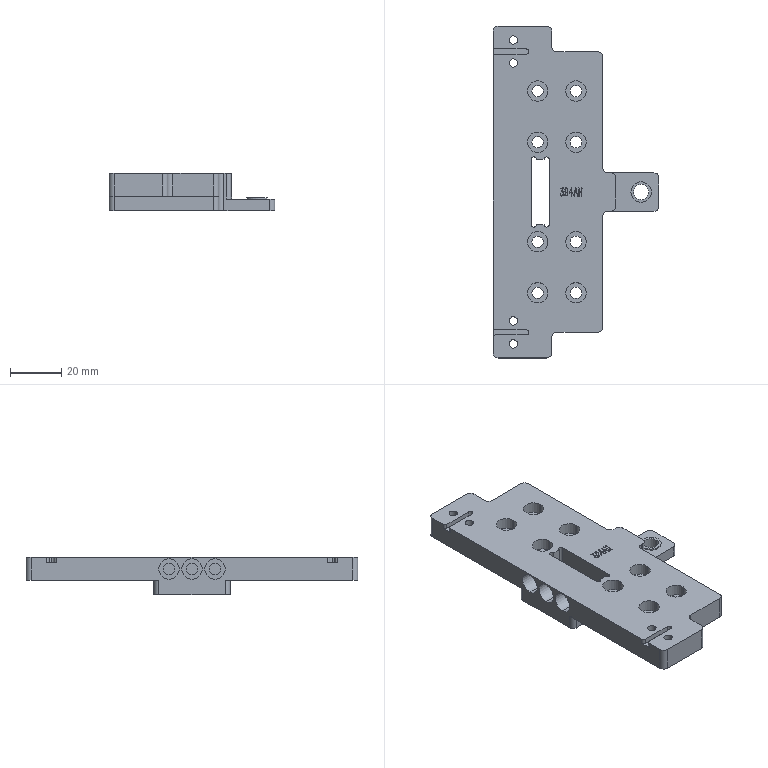NC program | NX | posted with a generic post | part box 65 x 130 x 14.5 mm
Lines 11007 to 11541 of 11541:
(PLANAR_MILL_COPY_COPY_COPY_COPY_COPY_COPY_1_COPY , TOOL : D6A45)
N21958 T01 M6
N21960 G54
N21962 G17 G0 G90 X-0.428 Y-26.291 B0. C0. S9500 M3
N21964 G43 Z30. H1
N21966 Z0.5
N21968 G94 G1 Z-1. F1250.
N21970 X-0.866 Y-27.1
N21972 G3 X0. Y-27.6 R1.
N21974 X2.1 Y-25.5 R2.1
N21976 X0. Y-27.6 R-2.1
N21978 X0.866 Y-27.1 R1.
N21980 G1 X0.428 Y-26.291
N21982 Z0.5
N21984 G0 Z30.
N21986 X-17.1 Y9.73
N21988 Z0.5
N21990 G1 Z-1.
N21992 X-16.4 Y10.134
N21994 G3 X-15.9 Y11. R1.
N21996 G1 Y30.5
N21998 G2 X-13. Y33.4 R2.9
N22000 G1 X13.
N22002 G2 X15.9 Y30.5 R2.9
N22004 G1 Y-8.5
N22006 G2 X13. Y-11.4 R2.9
N22008 G1 X9.5
N22010 G3 X8.4 Y-12.5 R1.1
N22012 G1 Y-30.5
N22014 G2 X5.5 Y-33.4 R2.9
N22016 G1 X-5.5
N22018 G2 X-8.4 Y-30.5 R2.9
N22020 G1 Y-12.5
N22022 G3 X-9.5 Y-11.4 R1.1
N22024 G1 X-13.
N22026 G2 X-15.9 Y-8.5 R2.9
N22028 G1 Y11.
N22030 G3 X-16.4 Y11.866 R1.
N22032 G1 X-17.1 Y12.27
N22034 Z0.5
N22036 G0 Z30.
N22038 X1.27 Y15.4
N22040 Z0.5
N22042 G1 Z-1.
N22044 X0.866 Y16.1
N22046 G3 X0. Y16.6 R1.
N22048 G1 X-12.75
N22050 G3 X-12.759 Y16.4 R0.1
N22052 G2 X-11.85 Y15.405 R1.
N22054 G1 Y12.595
N22056 G2 X-12.759 Y11.6 R1.
N22058 G3 X-12.75 Y11.4 R0.1
N22060 G1 X12.75
N22062 G3 X12.759 Y11.6 R0.1
N22064 G2 X11.85 Y12.595 R1.
N22066 G1 Y15.405
N22068 G2 X12.759 Y16.4 R1.
N22070 G3 X12.75 Y16.6 R0.1
N22072 G1 X0.
N22074 G3 X-0.866 Y16.1 R1.
N22076 G1 X-1.27 Y15.4
N22078 Z0.5
N22080 G0 Z30.
(PLANAR_MILL_COPY_COPY_COPY_COPY_COPY_COPY_1_COPY_COPY , TOOL : D6A45)
N22082 X59.924 Y23.874
N22084 Z-5.
N22086 G1 X60.052 Y23.948 Z-5.04
N22088 X60.25 Y24.286 Z-5.144
N22090 Y24.714 Z-5.259
N22092 X60.052 Y25.052 Z-5.364
N22094 X59.714 Y25.25 Z-5.469
N22096 X59.286 Z-5.584
N22098 X58.948 Y25.052 Z-5.689
N22100 X58.75 Y24.714 Z-5.794
N22102 Y24.286 Z-5.908
N22104 X58.948 Y23.948 Z-6.013
N22106 X59.286 Y23.75 Z-6.118
N22108 X59.714 Z-6.233
N22110 X60.052 Y23.948 Z-6.338
N22112 X60.25 Y24.286 Z-6.443
N22114 Y24.5 Z-6.5
N22116 G3 X59.5 Y25.25 R0.75
N22118 X60.25 Y24.5 R-0.75
N22120 X60. Y24.933 R0.5
N22122 G1 Z-5.
N22124 G0 Z30.
N22126 X51.126 Y24.924
N22128 Z-5.
N22130 G1 X51.052 Y25.052 Z-5.04
N22132 X50.714 Y25.25 Z-5.144
N22134 X50.286 Z-5.259
N22136 X49.948 Y25.052 Z-5.364
N22138 X49.75 Y24.714 Z-5.469
N22140 Y24.286 Z-5.584
N22142 X49.948 Y23.948 Z-5.689
N22144 X50.286 Y23.75 Z-5.794
N22146 X50.714 Z-5.908
N22148 X51.052 Y23.948 Z-6.013
N22150 X51.25 Y24.286 Z-6.118
N22152 Y24.714 Z-6.233
N22154 X51.052 Y25.052 Z-6.338
N22156 X50.714 Y25.25 Z-6.443
N22158 X50.5 Z-6.5
N22160 G3 X49.75 Y24.5 R0.75
N22162 X50.5 Y25.25 R-0.75
N22164 X50.067 Y25. R0.5
N22166 G1 Z-5.
N22168 G0 Z30.
N22170 X17.963 Y35.
N22172 Z-5.
N22174 G1 Z-6.5
N22176 X17.642 Y34.399
N22178 G3 X17.673 Y33.4 R1.
N22180 G1 X63.
N22182 G2 X65.9 Y30.5 R2.9
N22184 G1 Y11.5
N22186 G2 X63. Y8.6 R2.9
N22188 G1 X57.
N22190 G3 X55.9 Y7.5 R1.1
N22192 G1 Y-8.5
N22194 G2 X53. Y-11.4 R2.9
N22196 G1 X43.1
N22198 G2 X42.1 Y-10.4 R1.
N22200 G1 Y29.5
N22202 X42.113 Y29.565
N22204 X42.065 Y29.613
N22206 X42. Y29.6
N22208 X18.5
N22210 G3 X19. Y28.734 R1.
N22212 G1 X19.7 Y28.33
N22214 Z-5.
N22216 G0 Z30.
N22218 X-19.7
N22220 Z-5.
N22222 G1 Z-6.5
N22224 X-19. Y28.734
N22226 G3 X-18.5 Y29.6 R1.
N22228 G1 X-42.
N22230 X-42.065 Y29.613
N22232 X-42.113 Y29.565
N22234 X-42.1 Y29.5
N22236 Y-10.4
N22238 G2 X-43.1 Y-11.4 R1.
N22240 G1 X-53.
N22242 G2 X-55.9 Y-8.5 R2.9
N22244 G1 Y7.5
N22246 G3 X-57. Y8.6 R1.1
N22248 G1 X-63.
N22250 G2 X-65.9 Y11.5 R2.9
N22252 G1 Y30.5
N22254 G2 X-63. Y33.4 R2.9
N22256 G1 X-17.673
N22258 G3 X-17.642 Y34.399 R1.
N22260 G1 X-17.963 Y35.
N22262 Z-5.
N22264 G0 Z30.
N22266 X-49.874 Y24.924
N22268 Z-5.
N22270 G1 X-49.948 Y25.052 Z-5.04
N22272 X-50.286 Y25.25 Z-5.144
N22274 X-50.714 Z-5.259
N22276 X-51.052 Y25.052 Z-5.364
N22278 X-51.25 Y24.714 Z-5.469
N22280 Y24.286 Z-5.584
N22282 X-51.052 Y23.948 Z-5.689
N22284 X-50.714 Y23.75 Z-5.794
N22286 X-50.286 Z-5.908
N22288 X-49.948 Y23.948 Z-6.013
N22290 X-49.75 Y24.286 Z-6.118
N22292 Y24.714 Z-6.233
N22294 X-49.948 Y25.052 Z-6.338
N22296 X-50.286 Y25.25 Z-6.443
N22298 X-50.5 Z-6.5
N22300 G3 X-51.25 Y24.5 R0.75
N22302 X-50.5 Y25.25 R-0.75
N22304 X-50.933 Y25. R0.5
N22306 G1 Z-5.
N22308 G0 Z30.
N22310 X-59.924 Y25.126
N22312 Z-5.
N22314 G1 X-60.052 Y25.052 Z-5.04
N22316 X-60.25 Y24.714 Z-5.144
N22318 Y24.286 Z-5.259
N22320 X-60.052 Y23.948 Z-5.364
N22322 X-59.714 Y23.75 Z-5.469
N22324 X-59.286 Z-5.584
N22326 X-58.948 Y23.948 Z-5.689
N22328 X-58.75 Y24.286 Z-5.794
N22330 Y24.714 Z-5.908
N22332 X-58.948 Y25.052 Z-6.013
N22334 X-59.286 Y25.25 Z-6.118
N22336 X-59.714 Z-6.233
N22338 X-60.052 Y25.052 Z-6.338
N22340 X-60.25 Y24.714 Z-6.443
N22342 Y24.5 Z-6.5
N22344 G3 X-59.5 Y23.75 R0.75
N22346 X-60.25 Y24.5 R-0.75
N22348 X-60. Y24.067 R0.5
N22350 G1 Z-5.
N22352 G0 Z30.
(PLANAR_MILL_COPY_COPY_COPY_COPY_COPY_COPY_1_COPY_COPY_COPY , TOOL : D6A45)
N22354 X-38.408 Y0.761
N22356 Z-7.5
N22358 G1 X-38.524 Y0.976 Z-7.565
N22360 X-39.214 Y1.35 Z-7.776
N22362 X-39.5 Z-7.852
N22364 X-39.214 Z-7.929
N22366 X-38.524 Y0.976 Z-8.139
N22368 X-38.15 Y0.286 Z-8.349
N22370 Y-0.286 Z-8.503
N22372 X-38.524 Y-0.976 Z-8.713
N22374 X-39.214 Y-1.35 Z-8.923
N22376 X-39.5 Z-9.
N22378 G3 X-38.15 Y0. R1.35
N22380 X-39.5 Y1.35 R1.35
N22382 X-39. Y0.484 R1.
N22384 G1 Z-7.5
N22386 G0 Z30.
N22388 X-38.408 Y15.761
N22390 Z-7.5
N22392 G1 X-38.524 Y15.976 Z-7.565
N22394 X-39.214 Y16.35 Z-7.776
N22396 X-39.5 Z-7.852
N22398 X-39.214 Z-7.929
N22400 X-38.524 Y15.976 Z-8.139
N22402 X-38.15 Y15.286 Z-8.349
N22404 Y14.714 Z-8.503
N22406 X-38.524 Y14.024 Z-8.713
N22408 X-39.214 Y13.65 Z-8.923
N22410 X-39.5 Z-9.
N22412 G3 X-38.15 Y15. R1.35
N22414 X-39.5 Y16.35 R1.35
N22416 X-39. Y15.484 R1.
N22418 G1 Z-7.5
N22420 G0 Z30.
N22422 X-19.328 Y13.65
N22424 Z-7.5
N22426 G1 X-19.786 Z-7.623
N22428 X-20.476 Y14.024 Z-7.833
N22430 X-20.85 Y14.714 Z-8.043
N22432 Y15.286 Z-8.197
N22434 X-20.476 Y15.976 Z-8.407
N22436 X-19.786 Y16.35 Z-8.617
N22438 X-19.214 Z-8.77
N22440 X-18.692 Y16.119 Z-8.923
N22442 X-18.5 Y15.907 Z-9.
N22444 G3 X-18.5 Y14.093 R-1.35
N22446 X-19. Y14.959 R1.
N22448 G1 Z-7.5
N22450 G0 Z30.
N22452 X-19.328 Y-1.35
N22454 Z-7.5
N22456 G1 X-19.786 Z-7.623
N22458 X-20.476 Y-0.976 Z-7.833
N22460 X-20.85 Y-0.286 Z-8.043
N22462 Y0.286 Z-8.197
N22464 X-20.476 Y0.976 Z-8.407
N22466 X-19.786 Y1.35 Z-8.617
N22468 X-19.214 Z-8.77
N22470 X-18.692 Y1.119 Z-8.923
N22472 X-18.5 Y0.907 Z-9.
N22474 G3 X-18.5 Y-0.907 R-1.35
N22476 X-19. Y-0.041 R1.
N22478 G1 Z-7.5
N22480 G0 Z30.
N22482 X-17.963 Y-13.
N22484 Z-7.5
N22486 G1 Z-9.
N22488 X-17.642 Y-12.399
N22490 G3 X-17.673 Y-11.4 R1.
N22492 G1 X-39.618
N22494 G3 X-39.357 Y-12.365 R1.
N22496 G1 X-38.908 Y-12.813
N22498 Z-7.5
N22500 G0 Z30.
N22502 X38.908
N22504 Z-7.5
N22506 G1 Z-9.
N22508 X39.357 Y-12.365
N22510 G3 X39.618 Y-11.4 R1.
N22512 G1 X17.673
N22514 G3 X17.642 Y-12.399 R1.
N22516 G1 X17.963 Y-13.
N22518 Z-7.5
N22520 G0 Z30.
N22522 X19.328 Y1.35
N22524 Z-7.5
N22526 G1 X19.786 Z-7.623
N22528 X20.476 Y0.976 Z-7.833
N22530 X20.85 Y0.286 Z-8.043
N22532 Y-0.286 Z-8.197
N22534 X20.476 Y-0.976 Z-8.407
N22536 X19.786 Y-1.35 Z-8.617
N22538 X19.214 Z-8.77
N22540 X18.692 Y-1.119 Z-8.923
N22542 X18.5 Y-0.907 Z-9.
N22544 G3 X18.5 Y0.907 R-1.35
N22546 X19. Y0.041 R1.
N22548 G1 Z-7.5
N22550 G0 Z30.
N22552 X19.328 Y16.35
N22554 Z-7.5
N22556 G1 X19.786 Z-7.623
N22558 X20.476 Y15.976 Z-7.833
N22560 X20.85 Y15.286 Z-8.043
N22562 Y14.714 Z-8.197
N22564 X20.476 Y14.024 Z-8.407
N22566 X19.786 Y13.65 Z-8.617
N22568 X19.214 Z-8.77
N22570 X18.692 Y13.881 Z-8.923
N22572 X18.5 Y14.093 Z-9.
N22574 G3 X18.5 Y15.907 R-1.35
N22576 X19. Y15.041 R1.
N22578 G1 Z-7.5
N22580 G0 Z30.
N22582 X38.408 Y14.239
N22584 Z-7.5
N22586 G1 X38.524 Y14.024 Z-7.565
N22588 X39.214 Y13.65 Z-7.776
N22590 X39.5 Z-7.852
N22592 X39.214 Z-7.929
N22594 X38.524 Y14.024 Z-8.139
N22596 X38.15 Y14.714 Z-8.349
N22598 Y15. Z-8.426
N22600 Y15.286 Z-8.503
N22602 X38.524 Y15.976 Z-8.713
N22604 X39.214 Y16.35 Z-8.923
N22606 X39.5 Z-9.
N22608 G3 X38.15 Y15. R1.35
N22610 X39.5 Y13.65 R1.35
N22612 X39. Y14.516 R1.
N22614 G1 Z-7.5
N22616 G0 Z30.
N22618 X38.408 Y-0.761
N22620 Z-7.5
N22622 G1 X38.524 Y-0.976 Z-7.565
N22624 X39.214 Y-1.35 Z-7.776
N22626 X39.5 Z-7.852
N22628 X39.214 Z-7.929
N22630 X38.524 Y-0.976 Z-8.139
N22632 X38.15 Y-0.286 Z-8.349
N22634 Y0. Z-8.426
N22636 Y0.286 Z-8.503
N22638 X38.524 Y0.976 Z-8.713
N22640 X39.214 Y1.35 Z-8.923
N22642 X39.5 Z-9.
N22644 G3 X38.15 Y0. R1.35
N22646 X39.5 Y-1.35 R1.35
N22648 X39. Y-0.484 R1.
N22650 G1 Z-7.5
N22652 G0 Z30.
(DRILLING_COPY_1_COPY_1_COPY , TOOL : D6A45)
N22654 X-59.5 Y24.5 S5000
N22656 G81 G98 Z-7.6 F350. R-2.5
N22658 X-50.5
N22660 X50.5
N22662 X59.5
N22664 G80
N22666 G0 X59.5 Y24.5 Z30.
N22668 M5
(TOOLCOMP3_COPY_1 , TOOL : D3)
N22670 T16 M6
N22672 G54
N22674 G17 G0 G90 X-10.6 Y15.35 B0. C0. S9500 M3
N22676 G43 Z30. H16
N22678 Z-0.917
N22680 G94 G1 Z-2.417 F1000.
N22682 G41 X-11.05 Y15.76 D16
N22684 G3 X-11.2 Y15.5 R0.3
N22686 G1 Y12.5 F1200.
N22688 G2 X-11.267 Y12.05 R1.55
N22690 G1 X11.267
N22692 G2 X11.2 Y12.5 R1.55
N22694 G1 Y15.5
N22696 G2 X11.268 Y15.953 R1.55
N22698 G1 X11.222 Y15.95
N22700 X-11.267
N22702 G2 X-11.2 Y15.5 R1.55
N22704 G3 X-11.05 Y15.24 R0.3
N22706 G1 X-10.6 Y14.98
N22708 G40
N22710 X-10.506 Y14.946
N22712 Z-0.917
N22714 G0 Z30.
N22716 X-10.6 Y15.35
N22718 Z-3.333
N22720 G1 Z-4.833 F1000.
N22722 G41 X-11.05 Y15.76
N22724 G3 X-11.2 Y15.5 R0.3
N22726 G1 Y12.5 F1200.
N22728 G2 X-11.267 Y12.05 R1.55
N22730 G1 X11.267
N22732 G2 X11.2 Y12.5 R1.55
N22734 G1 Y15.5
N22736 G2 X11.268 Y15.953 R1.55
N22738 G1 X11.222 Y15.95
N22740 X-11.267
N22742 G2 X-11.2 Y15.5 R1.55
N22744 G3 X-11.05 Y15.24 R0.3
N22746 G1 X-10.6 Y14.98
N22748 G40
N22750 X-10.506 Y14.946
N22752 Z-3.333
N22754 G0 Z30.
N22756 X-10.6 Y15.35
N22758 Z-5.75
N22760 G1 Z-7.25 F1000.
N22762 G41 X-11.05 Y15.76
N22764 G3 X-11.2 Y15.5 R0.3
N22766 G1 Y12.5 F1200.
N22768 G2 X-11.267 Y12.05 R1.55
N22770 G1 X11.267
N22772 G2 X11.2 Y12.5 R1.55
N22774 G1 Y15.5
N22776 G2 X11.267 Y15.952 R1.55
N22778 G1 X11.222 Y15.95
N22780 X-11.267
N22782 G2 X-11.2 Y15.5 R1.55
N22784 G3 X-11.05 Y15.24 R0.3
N22786 G1 X-10.6 Y14.98
N22788 G40
N22790 X-10.506 Y14.946
N22792 Z-5.75
N22794 G0 Z30.
N22796 X-10.6 Y15.35
N22798 Z-8.167
N22800 G1 Z-9.667 F1000.
N22802 G41 X-11.05 Y15.76
N22804 G3 X-11.2 Y15.5 R0.3
N22806 G1 Y12.5 F1200.
N22808 G2 X-11.267 Y12.05 R1.55
N22810 G1 X11.267
N22812 G2 X11.2 Y12.5 R1.55
N22814 G1 Y15.5
N22816 G2 X11.267 Y15.951 R1.55
N22818 G1 X11.222 Y15.95
N22820 X-11.267
N22822 G2 X-11.2 Y15.5 R1.55
N22824 G3 X-11.05 Y15.24 R0.3
N22826 G1 X-10.6 Y14.98
N22828 G40
N22830 X-10.506 Y14.946
N22832 Z-8.167
N22834 G0 Z30.
N22836 X-10.6 Y15.35
N22838 Z-10.583
N22840 G1 Z-12.083 F1000.
N22842 G41 X-11.05 Y15.76
N22844 G3 X-11.2 Y15.5 R0.3
N22846 G1 Y12.5 F1200.
N22848 G2 X-11.267 Y12.05 R1.55
N22850 G1 X11.267
N22852 G2 X11.2 Y12.5 R1.55
N22854 G1 Y15.5
N22856 G2 X11.267 Y15.951 R1.55
N22858 G1 X11.236 Y15.95
N22860 X-11.267
N22862 G2 X-11.2 Y15.5 R1.55
N22864 G3 X-11.05 Y15.24 R0.3
N22866 G1 X-10.6 Y14.98
N22868 G40
N22870 X-10.506 Y14.946
N22872 Z-10.583
N22874 G0 Z30.
N22876 X-10.6 Y15.35
N22878 Z-13.
N22880 G1 Z-14.5 F1000.
N22882 G41 X-11.05 Y15.76
N22884 G3 X-11.2 Y15.5 R0.3
N22886 G1 Y12.5 F1200.
N22888 G2 X-11.267 Y12.05 R1.55
N22890 G1 X11.267
N22892 G2 X11.2 Y12.5 R1.55
N22894 G1 Y15.5
N22896 G2 X11.267 Y15.95 R1.55
N22898 G1 X11.236
N22900 X-11.267
N22902 G2 X-11.2 Y15.5 R1.55
N22904 G3 X-11.05 Y15.24 R0.3
N22906 G1 X-10.6 Y14.98
N22908 G40
N22910 X-10.506 Y14.946
N22912 Z-13.
N22914 G0 Z30.
N22916 M5
(TOOLCOMP111 , TOOL : D4)
N22918 T11 M6
N22920 G54
N22922 G17 G0 G90 X-12.892 Y-14.148 B0. C0. S9500 M3
N22924 G43 Z30. H11
N22926 Z-6.5
N22928 G94 G1 Z-8. F1250.
N22930 G41 X-12.91 Y-14.05 D11
N22932 X-13.388 Y-12.746
N22934 G3 X-13.695 Y-12.49 R0.4
N22936 G2 X-17.05 Y-8.5 R4.05
N22938 G1 Y28.45
N22940 X-40.95
N22942 Y-12.5
N22944 G3 X-40.75 Y-12.846 R0.4
N22946 G1 X-39.45 Y-13.597
N22948 G40
N22950 X-39.356 Y-13.631
N22952 Z-6.5
N22954 G0 Z30.
N22956 X39.356
N22958 Z-6.5
N22960 G1 Z-8.
N22962 G41 X39.45 Y-13.597
N22964 X40.75 Y-12.846
N22966 G3 X40.95 Y-12.5 R0.4
N22968 G1 Y28.45
N22970 X17.05
N22972 Y-8.5
N22974 G2 X13.695 Y-12.49 R4.05
N22976 G3 X13.388 Y-12.746 R0.4
N22978 G1 X12.91 Y-14.05
N22980 G40
N22982 X12.892 Y-14.148
N22984 Z-6.5
N22986 G0 Z30.
N22988 M5
N22990 M2